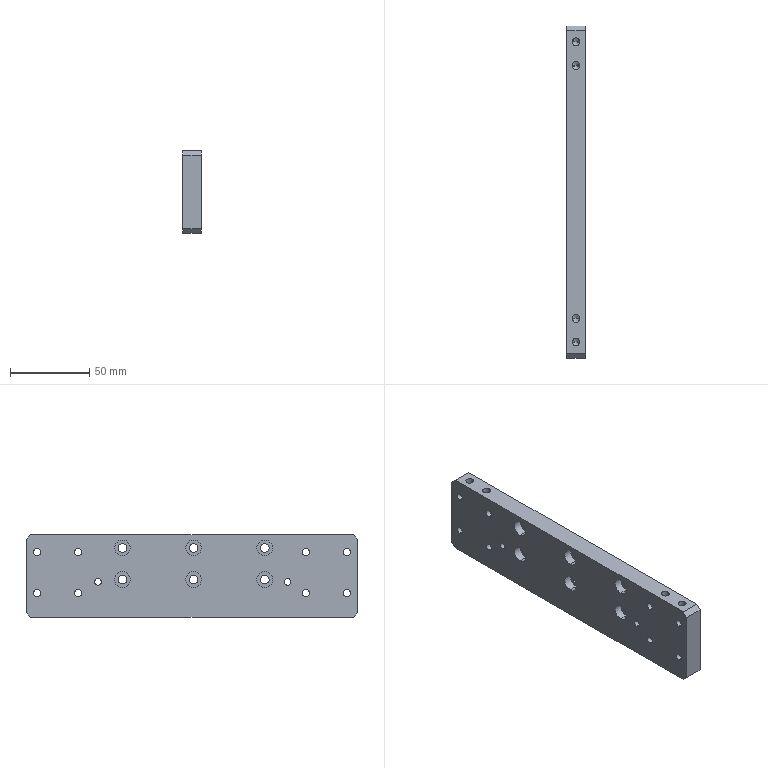Part | SolidWorks | features LPattern 5, HoleWzd 4, ICE 2, Chamfer 1, Extrusion 1, MirrorPattern 1 | 1 solid | 76 faces | box 12 x 210 x 52.5 mm | volume 125690 mm3 | cylinder 52 | plane 16 | cone 8 | commonest cylinder face diameters 4.5 x16 5.5 x12 10 x12 5 x8 4.2 x4